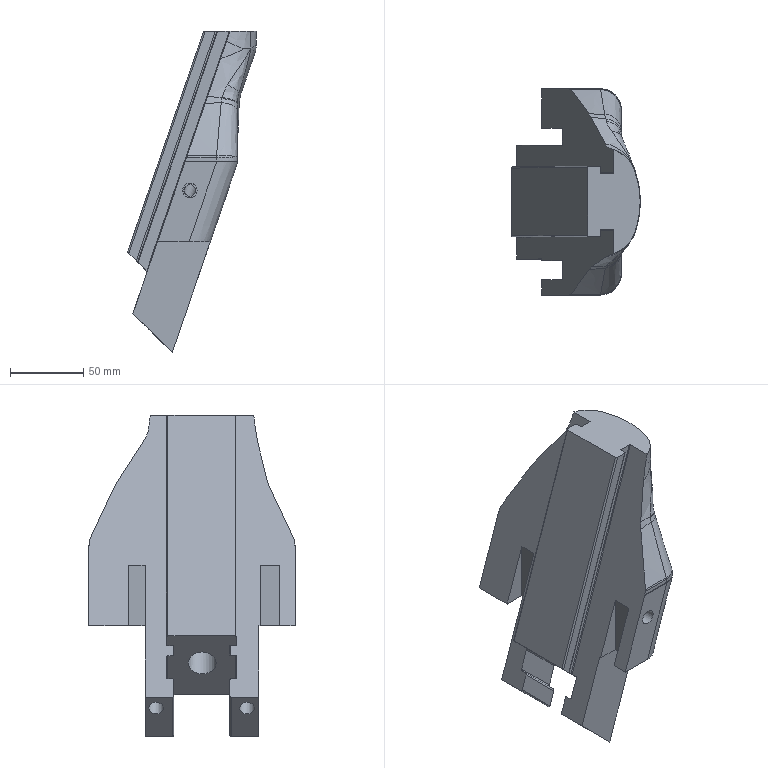Part | STEP file | solid 169 | 1 solid | 132 faces | box 87.731 x 140.677 x 218.816 mm | volume 678741 mm3 | spline 49 | plane 42 | cylinder 29 | cone 7 | other 5 | commonest cylinder face diameters 2 x12 8 x6 1 x4 10 x3 25 x2 16 x1